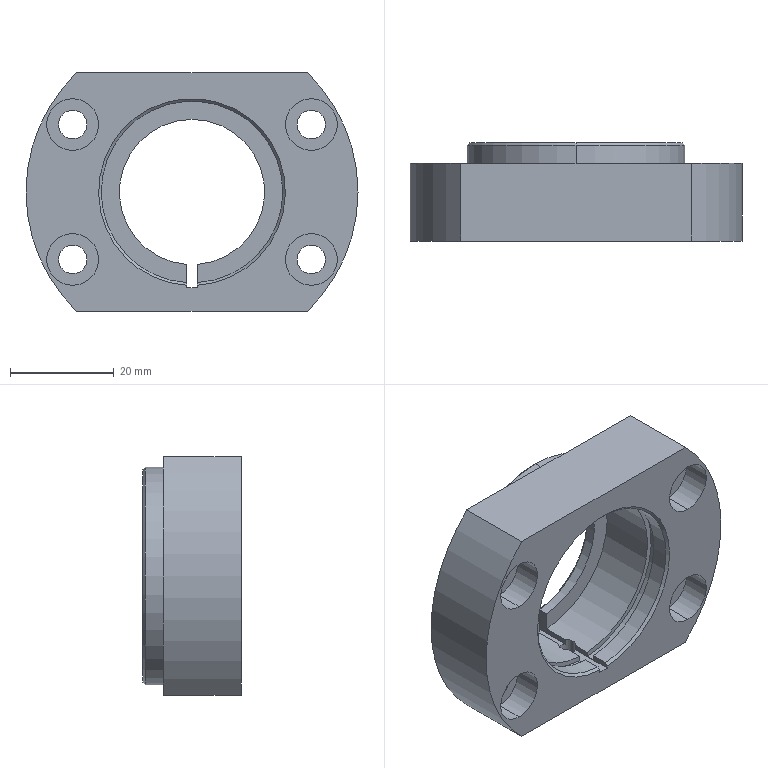Part | STEP file | ND25021-01-JDKM-01-GJ | 1 solid | 51 faces | box 64 x 19 x 46 mm | volume 25181 mm3 | cylinder 28 | plane 18 | cone 5 | commonest cylinder face diameters 5.5 x8 10 x8 3.3 x2 28 x2 35 x2 37 x2